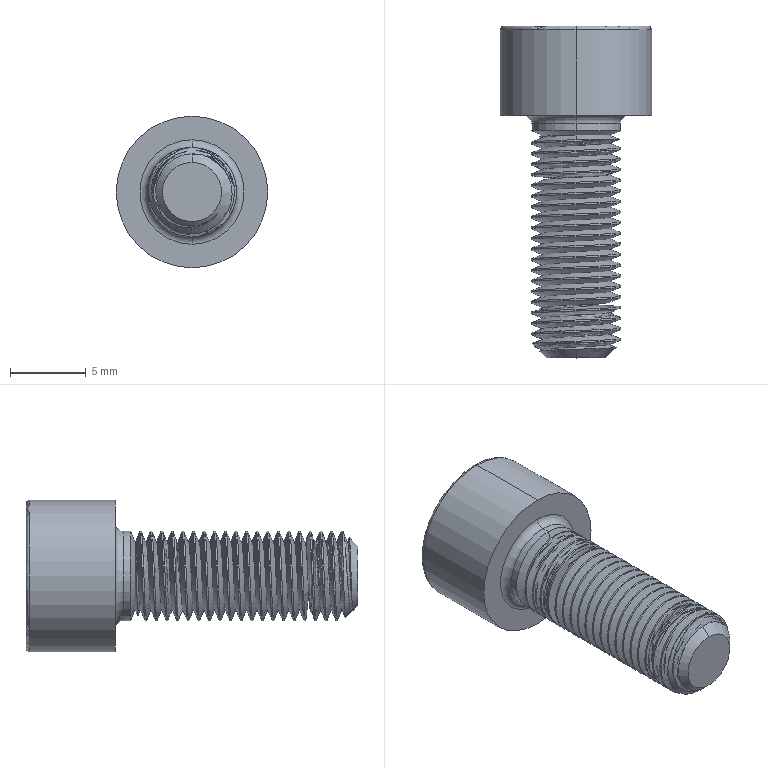Part | STEP file | Parafuso M6 - 16mm | 1 solid | 75 faces | box 10 x 21.9 x 10 mm | volume 696.612 mm3 | cylinder 44 | cone 13 | plane 10 | torus 6 | spline 2 | commonest cylinder face diameters 5.9 x42 10 x2